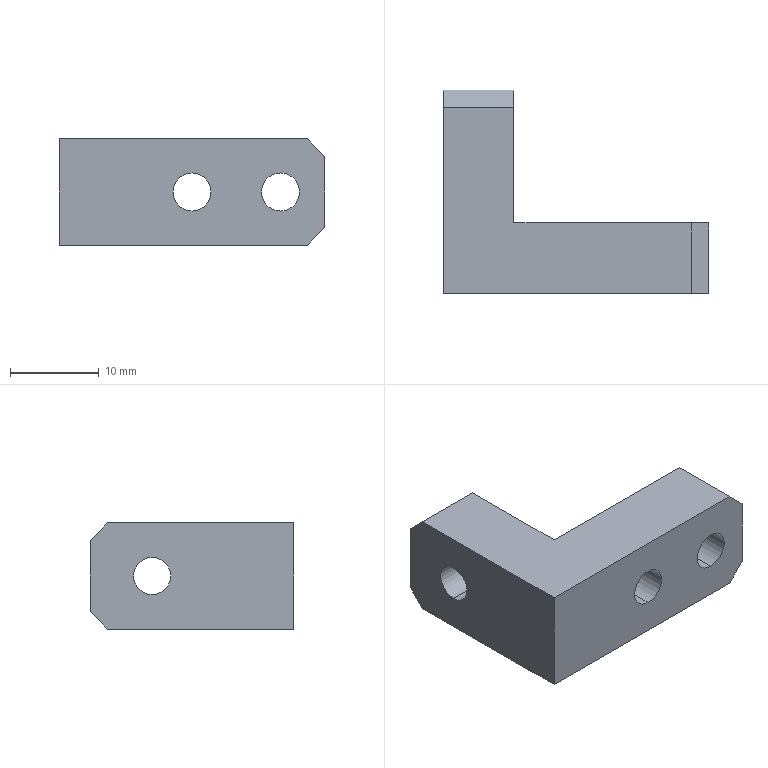Part | STEP file | PN_0056 Mount electronic clip limit mounting block B | 1 solid | 24 faces | box 30 x 23 x 12 mm | volume 3584 mm3 | plane 14 | cylinder 10 | commonest cylinder face diameters 4.3 x4 8 x4 4.2 x2